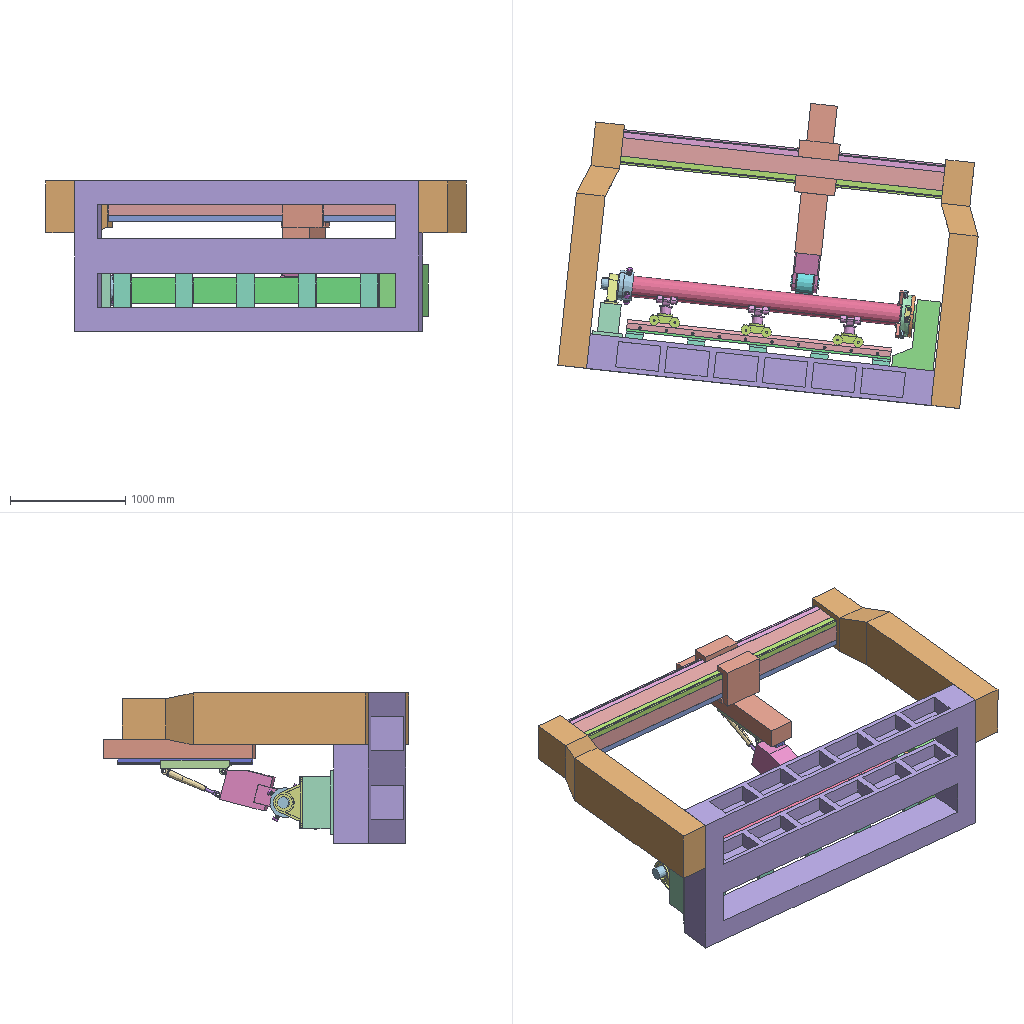Assembly | SolidWorks | 38 different items | 83 placed | box 3641 x 2643 x 1300 mm
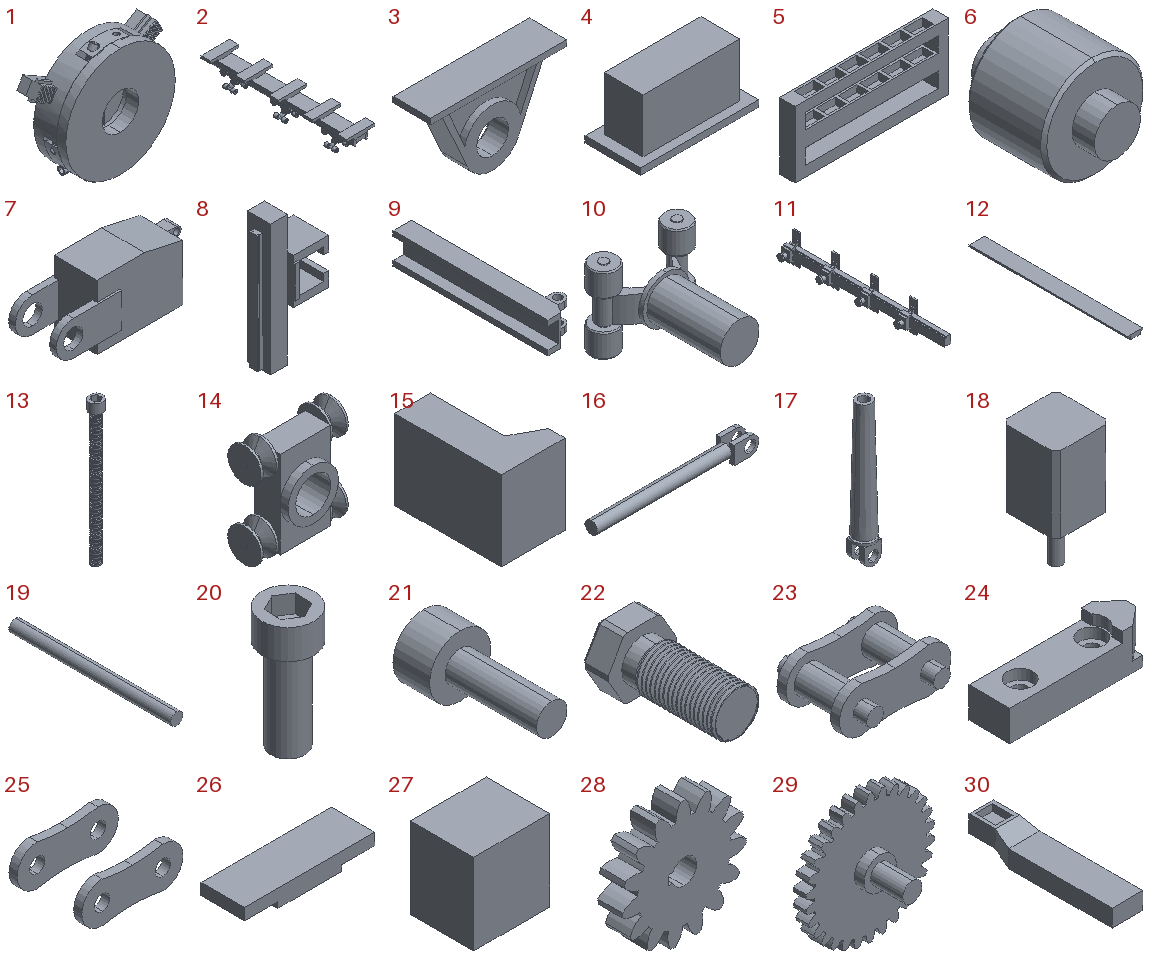Parts list (item | name | quantity | parent item | size | volume | features):
1 | (subassembly) | x1 | - | 422.408 x 144 x 419.924 mm | 8918159 mm3 | features ReferencePattern 12, LocalCirPattern 4, CompositeCurve 3, Cut 1
2 | (subassembly) | x1 | - | 450 x 2300 x 395.088 mm | 64996675 mm3 | features ReferencePattern 27, LocalLPattern 3, MirrorCompFeat 1
3 | - | x1 | - | 430 x 120 x 260 mm | 3516427 mm3 | features ICE 5, Extrusion 1, MirrorPattern 1
4 | - | x1 | - | 550 x 260 x 280 mm | 24540000 mm3 | features Extrusion 1, ICE 1
5 | - | x1 | - | 3000 x 300 x 1300 mm | 428496000 mm3 | features ICE 2, MirrorPattern 2, Extrusion 1
6 | - | x1 | - | 200 x 240 x 200 mm | 5312886 mm3 | features Chamfer 1, Extrusion 1, ICE 1
7 | - | x1 | - | 662 x 220 x 300 mm | 25140960 mm3 | features ICE 4, Extrusion 1, MirrorPattern 1
8 | - | x1 | - | 571 x 380 x 1300 mm | 81618000 mm3 | features ICE 4, Extrusion 1
9 | - | x1 | - | 125 x 600 x 120 mm | 3208933 mm3 | features ICE 4, MirrorPattern 2, Extrusion 1
10 | - | x3 | in 2 | 231 x 260.5 x 180 mm | 2038334 mm3 | features ICE 5, MirrorPattern 2, Extrusion 1, RefAxis 1, Revolution 1
11 | - | x1 | - | 260 x 2370 x 450 mm | 36834096 mm3 | features ICE 9, LPattern 3, Extrusion 1, MirrorPattern 1
12 | - | x1 | in 2 | 220 x 2300 x 60 mm | 22970661 mm3 | features Extrusion 1, HoleWzd 1, LPattern 1, MirrorPattern 1
13 | - | x3 | in 1 | 24.5 x 24.5 x 266.5 mm | 45236 mm3 | features ICE 2, Extrusion 1, Helix 1, Sweep 1
14 | - | x3 | in 2 | 229 x 108 x 266 mm | 2286238 mm3 | features ICE 6, LPattern 2, MirrorPattern 2, Revolution 1
15 | - | x1 | - | 360 x 600 x 450 mm | 64420319 mm3 | features ICE 3, Extrusion 1
16 | - | x1 | - | 356.143 x 40 x 40 mm | 216389 mm3 | features Extrusion 1, ICE 1, MirrorPattern 1
17 | - | x1 | - | 59.866 x 59.866 x 414.086 mm | 604728 mm3 | features Extrusion 1, MirrorPattern 1, Revolution 1
18 | - | x1 | - | 180 x 180 x 400 mm | 8211546 mm3 | features ICE 2, Chamfer 1, Extrusion 1
19 | - | x1 | - | 180 x 2400 x 180 mm | 61072561 mm3 | features Extrusion 1
20 | - | x6 | in 1 | 23 x 23 x 53 mm | 11275 mm3 | features ICE 2, Extrusion 1
21 | - | x20 | in 2 | 20 x 42 x 20 mm | 5300 mm3 | features ICE 2, Extrusion 1
22 | - | x4 | - | 49.962 x 90 x 45 mm | 85439 mm3 | features ICE 4, Chamfer 2, Extrusion 1, Helix 1, Sweep 1
23 | - | x1 | - | 100 x 80 x 40 mm | 102371 mm3 | features ICE 2, LPattern 2, RefPoint 2, Extrusion 1
24 | - | x3 | in 1 | 138 x 40 x 40 mm | 148074 mm3 | features ICE 5, Extrusion 1
25 | - | x1 | - | 100 x 72 x 40 mm | 48964 mm3 | features Extrusion 1, LPattern 1
26 | - | x5 | in 2 | 450 x 150 x 60 mm | 3360000 mm3 | features Extrusion 1
27 | - | x1 | - | 300 x 250 x 320 mm | 24000000 mm3 | features Extrusion 1
28 | - | x1 | - | 199.536 x 40 x 198.904 mm | 944330 mm3 | features Extrusion 1
29 | - | x1 | - | 398.808 x 170 x 400 mm | 5023065 mm3 | features ICE 2, Extrusion 1
30 | - | x2 | - | 450 x 2130 x 350 mm | 219500000 mm3 | features ICE 2, Extrusion 1
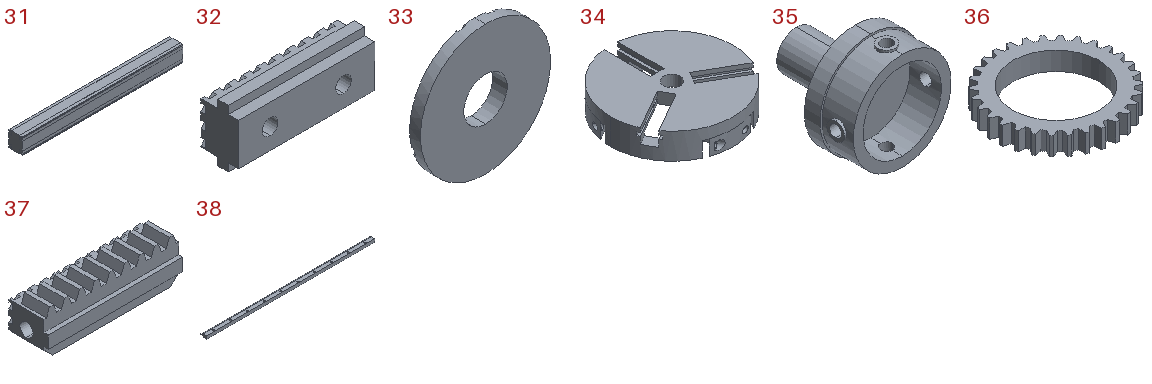31 | - | x1 | - | 3000 x 250 x 300 mm | 221738400 mm3 | features ICE 2, MirrorSolid 2, Extrusion 1
32 | - | x3 | in 1 | 130 x 36 x 55 mm | 187451 mm3 | features ICE 5, Extrusion 1
33 | - | x1 | in 1 | 360 x 40 x 360 mm | 2695575 mm3 | features ICE 2, CirPattern 1, Extrusion 1
34 | - | x1 | in 1 | 360 x 360 x 76 mm | 3930105 mm3 | features ICE 10, CirPattern 5, Cut 1, Extrusion 1
35 | - | x1 | - | 260 x 270 x 260 mm | 4719185 mm3 | features ICE 5, CirPattern 2, Extrusion 1
36 | - | x1 | in 1 | 199.365 x 200 x 30 mm | 379825 mm3 | features Extrusion 1
37 | - | x3 | in 1 | 162 x 47 x 52 mm | 270321 mm3 | features ICE 4, Chamfer 1, Extrusion 1
38 | - | x2 | in 2 | 2300 x 80 x 40 mm | 6073150 mm3 | features ICE 2, Extrusion 1, LPattern 1
Mates (type | each side: item.copy, entity, surface, feature):
In the top assembly
Coincident | 31.1 face plane Boss-Extrude1 | 30.1 face plane Cut-Extrude2 | 4 times
Coincident | 30.1 face plane Boss-Extrude1 | assembly plane
Coincident | 31.1 face plane Boss-Extrude1 | 30.2 face plane Cut-Extrude2 | 3 times
Coincident | 30.2 face plane Cut-Extrude1 | 5.1 face plane Boss-Extrude1
Coincident | 30.1 face plane Cut-Extrude1 | 5.1 face plane Boss-Extrude1
Coincident | 30.2 face plane Boss-Extrude1 | 5.1 face plane Boss-Extrude1 | 2 times
Coincident | 5.1 face plane Boss-Extrude1 | 15.1 face plane Boss-Extrude1
Concentric | 19.1 face cylinder Boss-Extrude1 | 35.1 face cylinder Boss-Extrude1
DistanceDim | 35.1 face plane Boss-Extrude2 | 19.1 face plane Boss-Extrude1
DistanceDim | 15.1 face plane Boss-Extrude1 | 5.1 face plane Boss-Extrude1
Concentric | 35.1 face cylinder Boss-Extrude3 | 3.1 face cylinder Boss-Extrude1
Coincident | 35.1 face plane Boss-Extrude4 | 3.1 face plane Boss-Extrude1
Parallel | 5.1 face plane Boss-Extrude1 | 3.1 face plane Boss-Extrude1
Concentric | 35.1 face cylinder Cut-Extrude1 | 22.1 face cylinder Boss-Extrude2
Tangent | 19.1 face cylinder Boss-Extrude1 | 22.1 face plane Cut-Extrude2
Coincident | 3.1 face plane Boss-Extrude1 | 4.1 face plane Boss-Extrude1
DistanceDim | 4.1 face plane Boss-Extrude1 | 3.1 face plane Boss-Extrude2 | 2 times
DistanceDim | 4.1 face plane Boss-Extrude2 | 5.1 face plane Boss-Extrude1
Coincident | 31.1 face plane Boss-Extrude1 | 8.1 face plane Boss-Extrude1 | 2 times
Coincident | 8.1 face plane Boss-Extrude4 | 9.1 face plane Boss-Extrude1 | 2 times
Concentric | 9.1 face cylinder Boss-Extrude2 | 7.1 face cylinder Boss-Extrude2
DistanceDim | 7.1 face plane Boss-Extrude2 | 9.1 face plane Boss-Extrude2
Concentric | 7.1 face cylinder Boss-Extrude3 | 6.1 face cylinder Boss-Extrude1
DistanceDim | 6.1 face plane Boss-Extrude2 | 7.1 face plane Boss-Extrude3
Concentric | 9.1 face cylinder Boss-Extrude3 | 17.1 face cylinder Mirror5
Coincident | 9.1 face plane Boss-Extrude3 | 17.1 face plane Boss-Extrude1
Concentric | 7.1 face cylinder Boss-Extrude4 | 16.1 face cylinder Boss-Extrude1
Concentric | 17.1 face cylinder Revolve1 | 16.1 face cylinder Boss-Extrude2
Parallel | 5.1 face plane Boss-Extrude1 | 12.1 face plane Boss-Extrude1
DistanceDim | 12.1 face plane Boss-Extrude1 | 15.1 face plane Boss-Extrude1
Concentric | 15.1 select_type:24 | 33.1 face cylinder Boss-Extrude1
Concentric | 19.1 face cylinder Boss-Extrude1 | 34.1 face cylinder Boss-Extrude1
Coincident | 15.1 face plane Boss-Extrude2 | 33.1 face plane Boss-Extrude1
DistanceDim | 19.1 face plane Boss-Extrude1 | 34.1 face plane Boss-Extrude1
Coincident | 5.1 face plane Boss-Extrude1 | 26.1 face plane Boss-Extrude1
In subassembly 2
Concentric | 12.2 face cylinder Tap Drill for M10 Tap1 | 38.1 face cylinder Cut-Extrude1
Concentric | 12.2 face cylinder LPattern1 | 38.1 face cylinder LPattern1
Coincident | 12.2 face plane Boss-Extrude1 | 38.1 face plane Boss-Extrude1
Concentric | 12.2 face cylinder Mirror1 | 38.2 face cylinder Cut-Extrude1
Concentric | 12.2 face cylinder Mirror1 | 38.2 face cylinder LPattern1
Coincident | 12.2 face plane Boss-Extrude1 | 38.2 face plane Boss-Extrude1
Concentric | 38.2 face cylinder Cut-Extrude1 | 21.1 face cylinder Boss-Extrude1
Coincident | 38.2 face plane Cut-Extrude2 | 21.1 face plane Boss-Extrude2
Tangent | 38.2 face plane Boss-Extrude1 | 14.1 face cylinder LPattern2
Tangent | 38.1 face plane Boss-Extrude1 | 14.1 face cylinder Revolve1
Concentric | 14.1 face cylinder Cut-Extrude2 | 10.1 face cylinder Boss-Extrude1
Parallel | 14.1 edge | 10.1 edge
DistanceDim | 14.1 face plane LPattern2 | 38.2 face plane Boss-Extrude1
Coincident | 12.2 face plane Boss-Extrude1 | 26.2 face plane Boss-Extrude1 | 3 times
Tangent | 10.1 face cylinder Mirror1 | 2.1 select_type:10
In subassembly 1
Concentric | 33.2 face cylinder Boss-Extrude1 | 36.1 face cylinder Boss-Extrude1
Coincident | 33.2 face plane Boss-Extrude1 | 36.1 face plane Boss-Extrude1
Coincident | 33.2 face plane Boss-Extrude1 | 37.1 face plane Boss-Extrude1
RackPinionDim | 37.1 select_type:24 | 36.1 select_type:24
Concentric | 37.1 edge | 13.1 face cylinder Boss-Extrude1
Parallel | 37.1 face plane Boss-Extrude1 | 1.1 plane
Screw | 37.1 face cylinder Cut-Extrude1 | 13.1 face cylinder Boss-Extrude1
Coincident | 33.2 face plane Cut-Extrude2 | 37.1 face plane Boss-Extrude3
Concentric | 33.2 face cylinder Boss-Extrude1 | 34.2 face cylinder Boss-Extrude1
Parallel | 37.1 face plane Boss-Extrude1 | 34.2 face plane Cut-Extrude1
DistanceDim | 34.2 face plane Boss-Extrude1 | 37.1 face plane Boss-Extrude2
Coincident | 32.1 face plane Boss-Extrude1 | 34.2 face plane Cut-Extrude1
Coincident | 37.1 face plane Cut-Extrude3 | 32.1 face plane Boss-Extrude1
Coincident | 37.1 face plane Cut-Extrude3 | 32.1 face plane Cut-Extrude2
LimitDistanceDim | 37.1 face plane Boss-Extrude1 | 34.2 face plane Boss-Extrude2
Coincident | 13.1 face plane Boss-Extrude2 | 34.2 face plane CirPattern7
Concentric | 32.1 face cylinder Cut-Extrude4 | 24.1 face cylinder Cut-Extrude2 | 2 times
Coincident | 32.1 face plane Boss-Extrude3 | 24.1 face plane Boss-Extrude1
Concentric | 24.1 face cylinder Cut-Extrude2 | 20.1 face cylinder Boss-Extrude1
Coincident | 24.1 face plane Cut-Extrude4 | 20.1 face plane Boss-Extrude2
Concentric | 24.1 face cylinder Cut-Extrude2 | 20.2 face cylinder Boss-Extrude1
Coincident | 24.1 face plane Cut-Extrude4 | 20.2 face plane Boss-Extrude2
Tangent | 24.1 face plane Boss-Extrude2 | 1.1 select_type:10